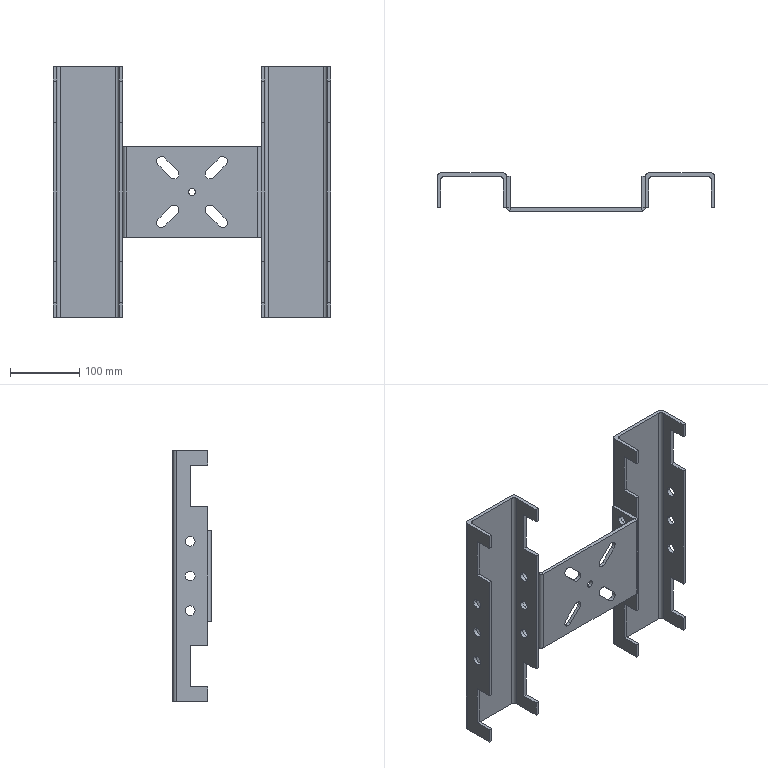Part | 3 solids | 140 faces | box 400 x 55 x 363 mm | volume 792088 mm3 | plane 78 | cylinder 62 | commonest cylinder face diameters 14 x48 10 x10 0.4 x2 10.4 x2